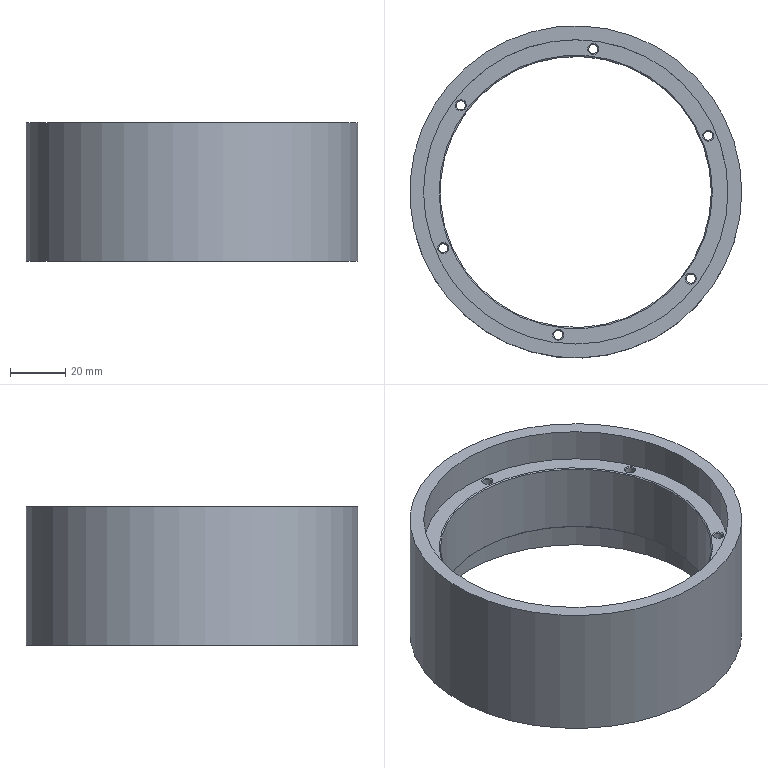Part | NX | features Instance Feature 6, SYMBOLIC_THREAD 6, DATUM_CSYS 5, IDENTICAL INSTANCE OUTPUT 5, EXTRUDE 4, SKETCH 4, EXTRACT_FACE 2, EXTRACT_STRING 2, CHAMFER 1, DATUM_PLANE 1, HOLE PACKAGE 1, MASTER SNAPSHOT BODY 1, Mirror Feature 1, Pattern Feature 1, SIMPLE HOLE 1 | 1 solid | 28 faces | box 120 x 120 x 50 mm | volume 139903 mm3 | cone 14 | cylinder 10 | plane 4 | commonest cylinder face diameters 3.3 x6 110 x2 98 x1 120 x1
STEP:
#1=CARTESIAN_POINT('',(60.,0.,-50.));
#2=VERTEX_POINT('',#1);
#3=CARTESIAN_POINT('',(0.,0.,-50.));
#4=DIRECTION('',(0.,0.,1.));
#5=DIRECTION('',(1.,0.,0.));
#6=AXIS2_PLACEMENT_3D('',#3,#4,#5);
#7=CIRCLE('',#6,60.);
#8=EDGE_CURVE('',#2,#2,#7,.T.);
#9=ORIENTED_EDGE('',*,*,#8,.T.);
#10=EDGE_LOOP('',(#9));
#11=FACE_BOUND('',#10,.T.);
#12=CARTESIAN_POINT('',(60.,0.,0.));
#13=VERTEX_POINT('',#12);
#14=CARTESIAN_POINT('',(0.,0.,0.));
#15=DIRECTION('',(0.,0.,1.));
#16=DIRECTION('',(1.,0.,0.));
#17=AXIS2_PLACEMENT_3D('',#14,#15,#16);
#18=CIRCLE('',#17,60.);
#19=EDGE_CURVE('',#13,#13,#18,.T.);
#20=ORIENTED_EDGE('',*,*,#19,.F.);
#21=EDGE_LOOP('',(#20));
#22=FACE_BOUND('',#21,.T.);
#23=CARTESIAN_POINT('',(0.,0.,-50.));
#24=DIRECTION('',(0.,0.,1.));
#25=DIRECTION('',(1.,0.,0.));
#26=AXIS2_PLACEMENT_3D('',#23,#24,#25);
#27=CYLINDRICAL_SURFACE('',#26,60.);
#28=ADVANCED_FACE('',(#11,#22),#27,.T.);
#29=CARTESIAN_POINT('',(55.,0.,-50.));
#30=VERTEX_POINT('',#29);
#31=CARTESIAN_POINT('',(0.,0.,-50.));
#32=DIRECTION('',(0.,0.,1.));
#33=DIRECTION('',(1.,0.,0.));
#34=AXIS2_PLACEMENT_3D('',#31,#32,#33);
#35=CIRCLE('',#34,55.);
#36=EDGE_CURVE('',#30,#30,#35,.T.);
#37=ORIENTED_EDGE('',*,*,#36,.T.);
#38=EDGE_LOOP('',(#37));
#39=FACE_BOUND('',#38,.T.);
#40=ORIENTED_EDGE('',*,*,#8,.F.);
#41=EDGE_LOOP('',(#40));
#42=FACE_BOUND('',#41,.T.);
#43=CARTESIAN_POINT('',(0.,0.,-50.));
#44=DIRECTION('',(0.,0.,1.));
#45=DIRECTION('',(1.,0.,0.));
#46=AXIS2_PLACEMENT_3D('',#43,#44,#45);
#47=PLANE('',#46);
#48=ADVANCED_FACE('',(#39,#42),#47,.F.);
#49=CARTESIAN_POINT('',(55.,0.,0.));
#50=VERTEX_POINT('',#49);
#51=CARTESIAN_POINT('',(0.,0.,0.));
#52=DIRECTION('',(0.,0.,1.));
#53=DIRECTION('',(1.,0.,0.));
#54=AXIS2_PLACEMENT_3D('',#51,#52,#53);
#55=CIRCLE('',#54,55.);
#56=EDGE_CURVE('',#50,#50,#55,.T.);
#57=ORIENTED_EDGE('',*,*,#56,.F.);
#58=EDGE_LOOP('',(#57));
#59=FACE_BOUND('',#58,.T.);
#60=ORIENTED_EDGE('',*,*,#19,.T.);
#61=EDGE_LOOP('',(#60));
#62=FACE_BOUND('',#61,.T.);
#63=CARTESIAN_POINT('',(0.,0.,0.));
#64=DIRECTION('',(0.,0.,1.));
#65=DIRECTION('',(1.,0.,0.));
#66=AXIS2_PLACEMENT_3D('',#63,#64,#65);
#67=PLANE('',#66);
#68=ADVANCED_FACE('',(#59,#62),#67,.T.);
#69=CARTESIAN_POINT('',(55.,0.,-12.));
#70=VERTEX_POINT('',#69);
#71=CARTESIAN_POINT('',(0.,0.,-12.));
#72=DIRECTION('',(0.,0.,1.));
#73=DIRECTION('',(1.,0.,0.));
#74=AXIS2_PLACEMENT_3D('',#71,#72,#73);
#75=CIRCLE('',#74,55.);
#76=EDGE_CURVE('',#70,#70,#75,.F.);
#77=ORIENTED_EDGE('',*,*,#76,.T.);
#78=EDGE_LOOP('',(#77));
#79=FACE_BOUND('',#78,.T.);
#80=ORIENTED_EDGE('',*,*,#56,.T.);
#81=EDGE_LOOP('',(#80));
#82=FACE_BOUND('',#81,.T.);
#83=CARTESIAN_POINT('',(0.,0.,-12.));
#84=DIRECTION('',(0.,0.,1.));
#85=DIRECTION('',(1.,0.,0.));
#86=AXIS2_PLACEMENT_3D('',#83,#84,#85);
#87=CYLINDRICAL_SURFACE('',#86,55.);
#88=ADVANCED_FACE('',(#79,#82),#87,.F.);
#89=CARTESIAN_POINT('',(49.38,0.,-12.));
#90=VERTEX_POINT('',#89);
#91=CARTESIAN_POINT('',(0.,0.,-12.));
#92=DIRECTION('',(0.,0.,1.));
#93=DIRECTION('',(1.,0.,0.));
#94=AXIS2_PLACEMENT_3D('',#91,#92,#93);
#95=CIRCLE('',#94,49.38);
#96=EDGE_CURVE('',#90,#90,#95,.F.);
#97=ORIENTED_EDGE('',*,*,#96,.T.);
#98=EDGE_LOOP('',(#97));
#99=FACE_BOUND('',#98,.T.);
#100=CARTESIAN_POINT('',(8.337,51.612,-12.));
#101=VERTEX_POINT('',#100);
#102=CARTESIAN_POINT('',(6.337,51.612,-12.));
#103=DIRECTION('',(0.,0.,1.));
#104=DIRECTION('',(1.,0.,0.));
#105=AXIS2_PLACEMENT_3D('',#102,#103,#104);
#106=CIRCLE('',#105,2.);
#107=EDGE_CURVE('',#101,#101,#106,.T.);
#108=ORIENTED_EDGE('',*,*,#107,.F.);
#109=EDGE_LOOP('',(#108));
#110=FACE_BOUND('',#109,.T.);
#111=CARTESIAN_POINT('',(49.866,20.318,-12.));
#112=VERTEX_POINT('',#111);
#113=CARTESIAN_POINT('',(47.866,20.318,-12.));
#114=DIRECTION('',(0.,0.,1.));
#115=DIRECTION('',(1.,0.,0.));
#116=AXIS2_PLACEMENT_3D('',#113,#114,#115);
#117=CIRCLE('',#116,2.);
#118=EDGE_CURVE('',#112,#112,#117,.T.);
#119=ORIENTED_EDGE('',*,*,#118,.F.);
#120=EDGE_LOOP('',(#119));
#121=FACE_BOUND('',#120,.T.);
#122=CARTESIAN_POINT('',(43.529,-31.294,-12.));
#123=VERTEX_POINT('',#122);
#124=CARTESIAN_POINT('',(41.529,-31.294,-12.));
#125=DIRECTION('',(0.,0.,1.));
#126=DIRECTION('',(1.,0.,0.));
#127=AXIS2_PLACEMENT_3D('',#124,#125,#126);
#128=CIRCLE('',#127,2.);
#129=EDGE_CURVE('',#123,#123,#128,.T.);
#130=ORIENTED_EDGE('',*,*,#129,.F.);
#131=EDGE_LOOP('',(#130));
#132=FACE_BOUND('',#131,.T.);
#133=CARTESIAN_POINT('',(-4.337,-51.612,-12.));
#134=VERTEX_POINT('',#133);
#135=CARTESIAN_POINT('',(-6.337,-51.612,-12.));
#136=DIRECTION('',(0.,0.,1.));
#137=DIRECTION('',(1.,0.,0.));
#138=AXIS2_PLACEMENT_3D('',#135,#136,#137);
#139=CIRCLE('',#138,2.);
#140=EDGE_CURVE('',#134,#134,#139,.T.);
#141=ORIENTED_EDGE('',*,*,#140,.F.);
#142=EDGE_LOOP('',(#141));
#143=FACE_BOUND('',#142,.T.);
#144=CARTESIAN_POINT('',(-45.866,-20.318,-12.));
#145=VERTEX_POINT('',#144);
#146=CARTESIAN_POINT('',(-47.866,-20.318,-12.));
#147=DIRECTION('',(0.,0.,1.));
#148=DIRECTION('',(1.,0.,0.));
#149=AXIS2_PLACEMENT_3D('',#146,#147,#148);
#150=CIRCLE('',#149,2.);
#151=EDGE_CURVE('',#145,#145,#150,.T.);
#152=ORIENTED_EDGE('',*,*,#151,.F.);
#153=EDGE_LOOP('',(#152));
#154=FACE_BOUND('',#153,.T.);
#155=CARTESIAN_POINT('',(-39.529,31.294,-12.));
#156=VERTEX_POINT('',#155);
#157=CARTESIAN_POINT('',(-41.529,31.294,-12.));
#158=DIRECTION('',(0.,0.,1.));
#159=DIRECTION('',(1.,0.,0.));
#160=AXIS2_PLACEMENT_3D('',#157,#158,#159);
#161=CIRCLE('',#160,2.);
#162=EDGE_CURVE('',#156,#156,#161,.T.);
#163=ORIENTED_EDGE('',*,*,#162,.F.);
#164=EDGE_LOOP('',(#163));
#165=FACE_BOUND('',#164,.T.);
#166=ORIENTED_EDGE('',*,*,#76,.F.);
#167=EDGE_LOOP('',(#166));
#168=FACE_BOUND('',#167,.T.);
#169=CARTESIAN_POINT('',(0.,0.,-12.));
#170=DIRECTION('',(0.,0.,1.));
#171=DIRECTION('',(1.,0.,0.));
#172=AXIS2_PLACEMENT_3D('',#169,#170,#171);
#173=PLANE('',#172);
#174=ADVANCED_FACE('',(#99,#110,#121,#132,#143,#154,#165,#168),#173,.T.);
#175=CARTESIAN_POINT('',(55.,0.,-38.));
#176=VERTEX_POINT('',#175);
#177=CARTESIAN_POINT('',(0.,0.,-38.));
#178=DIRECTION('',(0.,0.,1.));
#179=DIRECTION('',(1.,0.,0.));
#180=AXIS2_PLACEMENT_3D('',#177,#178,#179);
#181=CIRCLE('',#180,55.);
#182=EDGE_CURVE('',#176,#176,#181,.F.);
#183=ORIENTED_EDGE('',*,*,#182,.F.);
#184=EDGE_LOOP('',(#183));
#185=FACE_BOUND('',#184,.T.);
#186=ORIENTED_EDGE('',*,*,#36,.F.);
#187=EDGE_LOOP('',(#186));
#188=FACE_BOUND('',#187,.T.);
#189=CARTESIAN_POINT('',(0.,0.,-38.));
#190=DIRECTION('',(0.,0.,-1.));
#191=DIRECTION('',(-1.,0.,0.));
#192=AXIS2_PLACEMENT_3D('',#189,#190,#191);
#193=CYLINDRICAL_SURFACE('',#192,55.);
#194=ADVANCED_FACE('',(#185,#188),#193,.F.);
#195=CARTESIAN_POINT('',(49.38,0.,-38.));
#196=VERTEX_POINT('',#195);
#197=CARTESIAN_POINT('',(0.,0.,-38.));
#198=DIRECTION('',(0.,0.,1.));
#199=DIRECTION('',(1.,0.,0.));
#200=AXIS2_PLACEMENT_3D('',#197,#198,#199);
#201=CIRCLE('',#200,49.38);
#202=EDGE_CURVE('',#196,#196,#201,.T.);
#203=ORIENTED_EDGE('',*,*,#202,.T.);
#204=EDGE_LOOP('',(#203));
#205=FACE_BOUND('',#204,.T.);
#206=CARTESIAN_POINT('',(8.337,51.612,-38.));
#207=VERTEX_POINT('',#206);
#208=CARTESIAN_POINT('',(6.337,51.612,-38.));
#209=DIRECTION('',(0.,0.,1.));
#210=DIRECTION('',(1.,0.,0.));
#211=AXIS2_PLACEMENT_3D('',#208,#209,#210);
#212=CIRCLE('',#211,2.);
#213=EDGE_CURVE('',#207,#207,#212,.T.);
#214=ORIENTED_EDGE('',*,*,#213,.T.);
#215=EDGE_LOOP('',(#214));
#216=FACE_BOUND('',#215,.T.);
#217=CARTESIAN_POINT('',(49.866,20.318,-38.));
#218=VERTEX_POINT('',#217);
#219=CARTESIAN_POINT('',(47.866,20.318,-38.));
#220=DIRECTION('',(0.,0.,1.));
#221=DIRECTION('',(1.,0.,0.));
#222=AXIS2_PLACEMENT_3D('',#219,#220,#221);
#223=CIRCLE('',#222,2.);
#224=EDGE_CURVE('',#218,#218,#223,.T.);
#225=ORIENTED_EDGE('',*,*,#224,.T.);
#226=EDGE_LOOP('',(#225));
#227=FACE_BOUND('',#226,.T.);
#228=CARTESIAN_POINT('',(43.529,-31.294,-38.));
#229=VERTEX_POINT('',#228);
#230=CARTESIAN_POINT('',(41.529,-31.294,-38.));
#231=DIRECTION('',(0.,0.,1.));
#232=DIRECTION('',(1.,0.,0.));
#233=AXIS2_PLACEMENT_3D('',#230,#231,#232);
#234=CIRCLE('',#233,2.);
#235=EDGE_CURVE('',#229,#229,#234,.T.);
#236=ORIENTED_EDGE('',*,*,#235,.T.);
#237=EDGE_LOOP('',(#236));
#238=FACE_BOUND('',#237,.T.);
#239=CARTESIAN_POINT('',(-4.337,-51.612,-38.));
#240=VERTEX_POINT('',#239);
#241=CARTESIAN_POINT('',(-6.337,-51.612,-38.));
#242=DIRECTION('',(0.,0.,1.));
#243=DIRECTION('',(1.,0.,0.));
#244=AXIS2_PLACEMENT_3D('',#241,#242,#243);
#245=CIRCLE('',#244,2.);
#246=EDGE_CURVE('',#240,#240,#245,.T.);
#247=ORIENTED_EDGE('',*,*,#246,.T.);
#248=EDGE_LOOP('',(#247));
#249=FACE_BOUND('',#248,.T.);
#250=CARTESIAN_POINT('',(-45.866,-20.318,-38.));
#251=VERTEX_POINT('',#250);
#252=CARTESIAN_POINT('',(-47.866,-20.318,-38.));
#253=DIRECTION('',(0.,0.,1.));
#254=DIRECTION('',(1.,0.,0.));
#255=AXIS2_PLACEMENT_3D('',#252,#253,#254);
#256=CIRCLE('',#255,2.);
#257=EDGE_CURVE('',#251,#251,#256,.T.);
#258=ORIENTED_EDGE('',*,*,#257,.T.);
#259=EDGE_LOOP('',(#258));
#260=FACE_BOUND('',#259,.T.);
#261=CARTESIAN_POINT('',(-39.529,31.294,-38.));
#262=VERTEX_POINT('',#261);
#263=CARTESIAN_POINT('',(-41.529,31.294,-38.));
#264=DIRECTION('',(0.,0.,1.));
#265=DIRECTION('',(1.,0.,0.));
#266=AXIS2_PLACEMENT_3D('',#263,#264,#265);
#267=CIRCLE('',#266,2.);
#268=EDGE_CURVE('',#262,#262,#267,.T.);
#269=ORIENTED_EDGE('',*,*,#268,.T.);
#270=EDGE_LOOP('',(#269));
#271=FACE_BOUND('',#270,.T.);
#272=ORIENTED_EDGE('',*,*,#182,.T.);
#273=EDGE_LOOP('',(#272));
#274=FACE_BOUND('',#273,.T.);
#275=CARTESIAN_POINT('',(0.,0.,-38.));
#276=DIRECTION('',(0.,0.,1.));
#277=DIRECTION('',(1.,0.,0.));
#278=AXIS2_PLACEMENT_3D('',#275,#276,#277);
#279=PLANE('',#278);
#280=ADVANCED_FACE('',(#205,#216,#227,#238,#249,#260,#271,#274),#279,.F.);
#281=CARTESIAN_POINT('',(49.,0.,-37.62));
#282=VERTEX_POINT('',#281);
#283=CARTESIAN_POINT('',(0.,0.,-37.62));
#284=DIRECTION('',(0.,0.,1.));
#285=DIRECTION('',(1.,0.,0.));
#286=AXIS2_PLACEMENT_3D('',#283,#284,#285);
#287=CIRCLE('',#286,49.);
#288=EDGE_CURVE('',#282,#282,#287,.F.);
#289=ORIENTED_EDGE('',*,*,#288,.T.);
#290=EDGE_LOOP('',(#289));
#291=FACE_BOUND('',#290,.T.);
#292=CARTESIAN_POINT('',(49.,0.,-12.38));
#293=VERTEX_POINT('',#292);
#294=CARTESIAN_POINT('',(0.,0.,-12.38));
#295=DIRECTION('',(0.,0.,1.));
#296=DIRECTION('',(1.,0.,0.));
#297=AXIS2_PLACEMENT_3D('',#294,#295,#296);
#298=CIRCLE('',#297,49.);
#299=EDGE_CURVE('',#293,#293,#298,.T.);
#300=ORIENTED_EDGE('',*,*,#299,.T.);
#301=EDGE_LOOP('',(#300));
#302=FACE_BOUND('',#301,.T.);
#303=CARTESIAN_POINT('',(0.,0.,-102.));
#304=DIRECTION('',(0.,0.,1.));
#305=DIRECTION('',(1.,0.,0.));
#306=AXIS2_PLACEMENT_3D('',#303,#304,#305);
#307=CYLINDRICAL_SURFACE('',#306,49.);
#308=ADVANCED_FACE('',(#291,#302),#307,.F.);
#309=CARTESIAN_POINT('',(-43.179,31.294,-37.65));
#310=VERTEX_POINT('',#309);
#311=CARTESIAN_POINT('',(-41.529,31.294,-37.65));
#312=DIRECTION('',(0.,0.,-1.));
#313=DIRECTION('',(-1.,0.,0.));
#314=AXIS2_PLACEMENT_3D('',#311,#312,#313);
#315=CIRCLE('',#314,1.65);
#316=EDGE_CURVE('',#310,#310,#315,.T.);
#317=ORIENTED_EDGE('',*,*,#316,.T.);
#318=EDGE_LOOP('',(#317));
#319=FACE_BOUND('',#318,.T.);
#320=CARTESIAN_POINT('',(-39.879,31.294,-12.35));
#321=VERTEX_POINT('',#320);
#322=CARTESIAN_POINT('',(-41.529,31.294,-12.35));
#323=DIRECTION('',(0.,0.,1.));
#324=DIRECTION('',(1.,0.,0.));
#325=AXIS2_PLACEMENT_3D('',#322,#323,#324);
#326=CIRCLE('',#325,1.65);
#327=EDGE_CURVE('',#321,#321,#326,.T.);
#328=ORIENTED_EDGE('',*,*,#327,.T.);
#329=EDGE_LOOP('',(#328));
#330=FACE_BOUND('',#329,.T.);
#331=CARTESIAN_POINT('',(-41.529,31.294,-12.));
#332=DIRECTION('',(0.,0.,-1.));
#333=DIRECTION('',(-1.,0.,0.));
#334=AXIS2_PLACEMENT_3D('',#331,#332,#333);
#335=CYLINDRICAL_SURFACE('',#334,1.65);
#336=ADVANCED_FACE('',(#319,#330),#335,.F.);
#337=ORIENTED_EDGE('',*,*,#162,.T.);
#338=EDGE_LOOP('',(#337));
#339=FACE_BOUND('',#338,.T.);
#340=ORIENTED_EDGE('',*,*,#327,.F.);
#341=EDGE_LOOP('',(#340));
#342=FACE_BOUND('',#341,.T.);
#343=CARTESIAN_POINT('',(-41.529,31.294,-14.));
#344=DIRECTION('',(0.,0.,1.));
#345=DIRECTION('',(1.,0.,0.));
#346=AXIS2_PLACEMENT_3D('',#343,#344,#345);
#347=CONICAL_SURFACE('',#346,0.,0.7854);
#348=ADVANCED_FACE('',(#339,#342),#347,.F.);
#349=ORIENTED_EDGE('',*,*,#316,.F.);
#350=EDGE_LOOP('',(#349));
#351=FACE_BOUND('',#350,.T.);
#352=ORIENTED_EDGE('',*,*,#268,.F.);
#353=EDGE_LOOP('',(#352));
#354=FACE_BOUND('',#353,.T.);
#355=CARTESIAN_POINT('',(-41.529,31.294,-36.));
#356=DIRECTION('',(0.,0.,-1.));
#357=DIRECTION('',(-1.,0.,0.));
#358=AXIS2_PLACEMENT_3D('',#355,#356,#357);
#359=CONICAL_SURFACE('',#358,0.,0.7854);
#360=ADVANCED_FACE('',(#351,#354),#359,.F.);
#361=CARTESIAN_POINT('',(4.687,51.612,-37.65));
#362=VERTEX_POINT('',#361);
#363=CARTESIAN_POINT('',(6.337,51.612,-37.65));
#364=DIRECTION('',(0.,0.,-1.));
#365=DIRECTION('',(-1.,0.,0.));
#366=AXIS2_PLACEMENT_3D('',#363,#364,#365);
#367=CIRCLE('',#366,1.65);
#368=EDGE_CURVE('',#362,#362,#367,.T.);
#369=ORIENTED_EDGE('',*,*,#368,.T.);
#370=EDGE_LOOP('',(#369));
#371=FACE_BOUND('',#370,.T.);
#372=CARTESIAN_POINT('',(7.987,51.612,-12.35));
#373=VERTEX_POINT('',#372);
#374=CARTESIAN_POINT('',(6.337,51.612,-12.35));
#375=DIRECTION('',(0.,0.,1.));
#376=DIRECTION('',(1.,0.,0.));
#377=AXIS2_PLACEMENT_3D('',#374,#375,#376);
#378=CIRCLE('',#377,1.65);
#379=EDGE_CURVE('',#373,#373,#378,.T.);
#380=ORIENTED_EDGE('',*,*,#379,.T.);
#381=EDGE_LOOP('',(#380));
#382=FACE_BOUND('',#381,.T.);
#383=CARTESIAN_POINT('',(6.337,51.612,-12.));
#384=DIRECTION('',(0.,0.,-1.));
#385=DIRECTION('',(-0.5,0.866,0.));
#386=AXIS2_PLACEMENT_3D('',#383,#384,#385);
#387=CYLINDRICAL_SURFACE('',#386,1.65);
#388=ADVANCED_FACE('',(#371,#382),#387,.F.);
#389=CARTESIAN_POINT('',(46.216,20.318,-37.65));
#390=VERTEX_POINT('',#389);
#391=CARTESIAN_POINT('',(47.866,20.318,-37.65));
#392=DIRECTION('',(0.,0.,-1.));
#393=DIRECTION('',(-1.,0.,0.));
#394=AXIS2_PLACEMENT_3D('',#391,#392,#393);
#395=CIRCLE('',#394,1.65);
#396=EDGE_CURVE('',#390,#390,#395,.T.);
#397=ORIENTED_EDGE('',*,*,#396,.T.);
#398=EDGE_LOOP('',(#397));
#399=FACE_BOUND('',#398,.T.);
#400=CARTESIAN_POINT('',(49.516,20.318,-12.35));
#401=VERTEX_POINT('',#400);
#402=CARTESIAN_POINT('',(47.866,20.318,-12.35));
#403=DIRECTION('',(0.,0.,1.));
#404=DIRECTION('',(1.,0.,0.));
#405=AXIS2_PLACEMENT_3D('',#402,#403,#404);
#406=CIRCLE('',#405,1.65);
#407=EDGE_CURVE('',#401,#401,#406,.T.);
#408=ORIENTED_EDGE('',*,*,#407,.T.);
#409=EDGE_LOOP('',(#408));
#410=FACE_BOUND('',#409,.T.);
#411=CARTESIAN_POINT('',(47.866,20.318,-12.));
#412=DIRECTION('',(0.,0.,-1.));
#413=DIRECTION('',(0.5,0.866,0.));
#414=AXIS2_PLACEMENT_3D('',#411,#412,#413);
#415=CYLINDRICAL_SURFACE('',#414,1.65);
#416=ADVANCED_FACE('',(#399,#410),#415,.F.);
#417=CARTESIAN_POINT('',(39.879,-31.294,-37.65));
#418=VERTEX_POINT('',#417);
#419=CARTESIAN_POINT('',(41.529,-31.294,-37.65));
#420=DIRECTION('',(0.,0.,-1.));
#421=DIRECTION('',(-1.,0.,0.));
#422=AXIS2_PLACEMENT_3D('',#419,#420,#421);
#423=CIRCLE('',#422,1.65);
#424=EDGE_CURVE('',#418,#418,#423,.T.);
#425=ORIENTED_EDGE('',*,*,#424,.T.);
#426=EDGE_LOOP('',(#425));
#427=FACE_BOUND('',#426,.T.);
#428=CARTESIAN_POINT('',(43.179,-31.294,-12.35));
#429=VERTEX_POINT('',#428);
#430=CARTESIAN_POINT('',(41.529,-31.294,-12.35));
#431=DIRECTION('',(0.,0.,1.));
#432=DIRECTION('',(1.,0.,0.));
#433=AXIS2_PLACEMENT_3D('',#430,#431,#432);
#434=CIRCLE('',#433,1.65);
#435=EDGE_CURVE('',#429,#429,#434,.T.);
#436=ORIENTED_EDGE('',*,*,#435,.T.);
#437=EDGE_LOOP('',(#436));
#438=FACE_BOUND('',#437,.T.);
#439=CARTESIAN_POINT('',(41.529,-31.294,-12.));
#440=DIRECTION('',(0.,0.,-1.));
#441=DIRECTION('',(1.,0.,0.));
#442=AXIS2_PLACEMENT_3D('',#439,#440,#441);
#443=CYLINDRICAL_SURFACE('',#442,1.65);
#444=ADVANCED_FACE('',(#427,#438),#443,.F.);
#445=CARTESIAN_POINT('',(-7.987,-51.612,-37.65));
#446=VERTEX_POINT('',#445);
#447=CARTESIAN_POINT('',(-6.337,-51.612,-37.65));
#448=DIRECTION('',(0.,0.,-1.));
#449=DIRECTION('',(-1.,0.,0.));
#450=AXIS2_PLACEMENT_3D('',#447,#448,#449);
#451=CIRCLE('',#450,1.65);
#452=EDGE_CURVE('',#446,#446,#451,.T.);
#453=ORIENTED_EDGE('',*,*,#452,.T.);
#454=EDGE_LOOP('',(#453));
#455=FACE_BOUND('',#454,.T.);
#456=CARTESIAN_POINT('',(-4.687,-51.612,-12.35));
#457=VERTEX_POINT('',#456);
#458=CARTESIAN_POINT('',(-6.337,-51.612,-12.35));
#459=DIRECTION('',(0.,0.,1.));
#460=DIRECTION('',(1.,0.,0.));
#461=AXIS2_PLACEMENT_3D('',#458,#459,#460);
#462=CIRCLE('',#461,1.65);
#463=EDGE_CURVE('',#457,#457,#462,.T.);
#464=ORIENTED_EDGE('',*,*,#463,.T.);
#465=EDGE_LOOP('',(#464));
#466=FACE_BOUND('',#465,.T.);
#467=CARTESIAN_POINT('',(-6.337,-51.612,-12.));
#468=DIRECTION('',(0.,0.,-1.));
#469=DIRECTION('',(0.5,-0.866,0.));
#470=AXIS2_PLACEMENT_3D('',#467,#468,#469);
#471=CYLINDRICAL_SURFACE('',#470,1.65);
#472=ADVANCED_FACE('',(#455,#466),#471,.F.);
#473=CARTESIAN_POINT('',(-49.516,-20.318,-37.65));
#474=VERTEX_POINT('',#473);
#475=CARTESIAN_POINT('',(-47.866,-20.318,-37.65));
#476=DIRECTION('',(0.,0.,-1.));
#477=DIRECTION('',(-1.,0.,0.));
#478=AXIS2_PLACEMENT_3D('',#475,#476,#477);
#479=CIRCLE('',#478,1.65);
#480=EDGE_CURVE('',#474,#474,#479,.T.);
#481=ORIENTED_EDGE('',*,*,#480,.T.);
#482=EDGE_LOOP('',(#481));
#483=FACE_BOUND('',#482,.T.);
#484=CARTESIAN_POINT('',(-46.216,-20.318,-12.35));
#485=VERTEX_POINT('',#484);
#486=CARTESIAN_POINT('',(-47.866,-20.318,-12.35));
#487=DIRECTION('',(0.,0.,1.));
#488=DIRECTION('',(1.,0.,0.));
#489=AXIS2_PLACEMENT_3D('',#486,#487,#488);
#490=CIRCLE('',#489,1.65);
#491=EDGE_CURVE('',#485,#485,#490,.T.);
#492=ORIENTED_EDGE('',*,*,#491,.T.);
#493=EDGE_LOOP('',(#492));
#494=FACE_BOUND('',#493,.T.);
#495=CARTESIAN_POINT('',(-47.866,-20.318,-12.));
#496=DIRECTION('',(0.,0.,-1.));
#497=DIRECTION('',(-0.5,-0.866,0.));
#498=AXIS2_PLACEMENT_3D('',#495,#496,#497);
#499=CYLINDRICAL_SURFACE('',#498,1.65);
#500=ADVANCED_FACE('',(#483,#494),#499,.F.);
#501=ORIENTED_EDGE('',*,*,#151,.T.);
#502=EDGE_LOOP('',(#501));
#503=FACE_BOUND('',#502,.T.);
#504=ORIENTED_EDGE('',*,*,#491,.F.);
#505=EDGE_LOOP('',(#504));
#506=FACE_BOUND('',#505,.T.);
#507=CARTESIAN_POINT('',(-47.866,-20.318,-14.));
#508=DIRECTION('',(0.,0.,1.));
#509=DIRECTION('',(1.,0.,0.));
#510=AXIS2_PLACEMENT_3D('',#507,#508,#509);
#511=CONICAL_SURFACE('',#510,0.,0.7854);
#512=ADVANCED_FACE('',(#503,#506),#511,.F.);
#513=ORIENTED_EDGE('',*,*,#140,.T.);
#514=EDGE_LOOP('',(#513));
#515=FACE_BOUND('',#514,.T.);
#516=ORIENTED_EDGE('',*,*,#463,.F.);
#517=EDGE_LOOP('',(#516));
#518=FACE_BOUND('',#517,.T.);
#519=CARTESIAN_POINT('',(-6.337,-51.612,-14.));
#520=DIRECTION('',(0.,0.,1.));
#521=DIRECTION('',(1.,0.,0.));
#522=AXIS2_PLACEMENT_3D('',#519,#520,#521);
#523=CONICAL_SURFACE('',#522,0.,0.7854);
#524=ADVANCED_FACE('',(#515,#518),#523,.F.);
#525=ORIENTED_EDGE('',*,*,#129,.T.);
#526=EDGE_LOOP('',(#525));
#527=FACE_BOUND('',#526,.T.);
#528=ORIENTED_EDGE('',*,*,#435,.F.);
#529=EDGE_LOOP('',(#528));
#530=FACE_BOUND('',#529,.T.);
#531=CARTESIAN_POINT('',(41.529,-31.294,-14.));
#532=DIRECTION('',(0.,0.,1.));
#533=DIRECTION('',(1.,0.,0.));
#534=AXIS2_PLACEMENT_3D('',#531,#532,#533);
#535=CONICAL_SURFACE('',#534,0.,0.7854);
#536=ADVANCED_FACE('',(#527,#530),#535,.F.);
#537=ORIENTED_EDGE('',*,*,#118,.T.);
#538=EDGE_LOOP('',(#537));
#539=FACE_BOUND('',#538,.T.);
#540=ORIENTED_EDGE('',*,*,#407,.F.);
#541=EDGE_LOOP('',(#540));
#542=FACE_BOUND('',#541,.T.);
#543=CARTESIAN_POINT('',(47.866,20.318,-14.));
#544=DIRECTION('',(0.,0.,1.));
#545=DIRECTION('',(1.,0.,0.));
#546=AXIS2_PLACEMENT_3D('',#543,#544,#545);
#547=CONICAL_SURFACE('',#546,0.,0.7854);
#548=ADVANCED_FACE('',(#539,#542),#547,.F.);
#549=ORIENTED_EDGE('',*,*,#107,.T.);
#550=EDGE_LOOP('',(#549));
#551=FACE_BOUND('',#550,.T.);
#552=ORIENTED_EDGE('',*,*,#379,.F.);
#553=EDGE_LOOP('',(#552));
#554=FACE_BOUND('',#553,.T.);
#555=CARTESIAN_POINT('',(6.337,51.612,-14.));
#556=DIRECTION('',(0.,0.,1.));
#557=DIRECTION('',(1.,0.,0.));
#558=AXIS2_PLACEMENT_3D('',#555,#556,#557);
#559=CONICAL_SURFACE('',#558,0.,0.7854);
#560=ADVANCED_FACE('',(#551,#554),#559,.F.);
#561=ORIENTED_EDGE('',*,*,#480,.F.);
#562=EDGE_LOOP('',(#561));
#563=FACE_BOUND('',#562,.T.);
#564=ORIENTED_EDGE('',*,*,#257,.F.);
#565=EDGE_LOOP('',(#564));
#566=FACE_BOUND('',#565,.T.);
#567=CARTESIAN_POINT('',(-47.866,-20.318,-36.));
#568=DIRECTION('',(0.,0.,-1.));
#569=DIRECTION('',(-1.,0.,0.));
#570=AXIS2_PLACEMENT_3D('',#567,#568,#569);
#571=CONICAL_SURFACE('',#570,0.,0.7854);
#572=ADVANCED_FACE('',(#563,#566),#571,.F.);
#573=ORIENTED_EDGE('',*,*,#246,.F.);
#574=EDGE_LOOP('',(#573));
#575=FACE_BOUND('',#574,.T.);
#576=ORIENTED_EDGE('',*,*,#452,.F.);
#577=EDGE_LOOP('',(#576));
#578=FACE_BOUND('',#577,.T.);
#579=CARTESIAN_POINT('',(-6.337,-51.612,-36.));
#580=DIRECTION('',(0.,0.,-1.));
#581=DIRECTION('',(-1.,0.,0.));
#582=AXIS2_PLACEMENT_3D('',#579,#580,#581);
#583=CONICAL_SURFACE('',#582,0.,0.7854);
#584=ADVANCED_FACE('',(#575,#578),#583,.F.);
#585=ORIENTED_EDGE('',*,*,#235,.F.);
#586=EDGE_LOOP('',(#585));
#587=FACE_BOUND('',#586,.T.);
#588=ORIENTED_EDGE('',*,*,#424,.F.);
#589=EDGE_LOOP('',(#588));
#590=FACE_BOUND('',#589,.T.);
#591=CARTESIAN_POINT('',(41.529,-31.294,-36.));
#592=DIRECTION('',(0.,0.,-1.));
#593=DIRECTION('',(-1.,0.,0.));
#594=AXIS2_PLACEMENT_3D('',#591,#592,#593);
#595=CONICAL_SURFACE('',#594,0.,0.7854);
#596=ADVANCED_FACE('',(#587,#590),#595,.F.);
#597=ORIENTED_EDGE('',*,*,#224,.F.);
#598=EDGE_LOOP('',(#597));
#599=FACE_BOUND('',#598,.T.);
#600=ORIENTED_EDGE('',*,*,#396,.F.);
#601=EDGE_LOOP('',(#600));
#602=FACE_BOUND('',#601,.T.);
#603=CARTESIAN_POINT('',(47.866,20.318,-36.));
#604=DIRECTION('',(0.,0.,-1.));
#605=DIRECTION('',(-1.,0.,0.));
#606=AXIS2_PLACEMENT_3D('',#603,#604,#605);
#607=CONICAL_SURFACE('',#606,0.,0.7854);
#608=ADVANCED_FACE('',(#599,#602),#607,.F.);
#609=ORIENTED_EDGE('',*,*,#213,.F.);
#610=EDGE_LOOP('',(#609));
#611=FACE_BOUND('',#610,.T.);
#612=ORIENTED_EDGE('',*,*,#368,.F.);
#613=EDGE_LOOP('',(#612));
#614=FACE_BOUND('',#613,.T.);
#615=CARTESIAN_POINT('',(6.337,51.612,-36.));
#616=DIRECTION('',(0.,0.,-1.));
#617=DIRECTION('',(-1.,0.,0.));
#618=AXIS2_PLACEMENT_3D('',#615,#616,#617);
#619=CONICAL_SURFACE('',#618,0.,0.7854);
#620=ADVANCED_FACE('',(#611,#614),#619,.F.);
#621=ORIENTED_EDGE('',*,*,#288,.F.);
#622=EDGE_LOOP('',(#621));
#623=FACE_BOUND('',#622,.T.);
#624=ORIENTED_EDGE('',*,*,#202,.F.);
#625=EDGE_LOOP('',(#624));
#626=FACE_BOUND('',#625,.T.);
#627=CARTESIAN_POINT('',(0.,0.,-38.));
#628=DIRECTION('',(0.,0.,-1.));
#629=DIRECTION('',(-1.,0.,0.));
#630=AXIS2_PLACEMENT_3D('',#627,#628,#629);
#631=CONICAL_SURFACE('',#630,49.38,0.7854);
#632=ADVANCED_FACE('',(#623,#626),#631,.F.);
#633=ORIENTED_EDGE('',*,*,#96,.F.);
#634=EDGE_LOOP('',(#633));
#635=FACE_BOUND('',#634,.T.);
#636=ORIENTED_EDGE('',*,*,#299,.F.);
#637=EDGE_LOOP('',(#636));
#638=FACE_BOUND('',#637,.T.);
#639=CARTESIAN_POINT('',(0.,0.,-12.38));
#640=DIRECTION('',(0.,0.,1.));
#641=DIRECTION('',(1.,0.,0.));
#642=AXIS2_PLACEMENT_3D('',#639,#640,#641);
#643=CONICAL_SURFACE('',#642,49.,0.7854);
#644=ADVANCED_FACE('',(#635,#638),#643,.F.);
#645=CLOSED_SHELL('',(#28,#48,#68,#88,#174,#194,#280,#308,#336,#348,#360,#388,#416,#444,#472,#500,#512,#524,#536,#548,#560,#572,#584,#596,#608,#620,#632,#644));
#646=MANIFOLD_SOLID_BREP('',#645);
#647=(LENGTH_UNIT()NAMED_UNIT(*)SI_UNIT(.MILLI.,.METRE.));
#648=UNCERTAINTY_MEASURE_WITH_UNIT(LENGTH_MEASURE(0.00001),#647,'','');
#649=(NAMED_UNIT(*)PLANE_ANGLE_UNIT()SI_UNIT($,.RADIAN.));
#650=(NAMED_UNIT(*)SI_UNIT($,.STERADIAN.)SOLID_ANGLE_UNIT());
#651=(GEOMETRIC_REPRESENTATION_CONTEXT(3)GLOBAL_UNCERTAINTY_ASSIGNED_CONTEXT((#648))GLOBAL_UNIT_ASSIGNED_CONTEXT((#647,#649,#650))REPRESENTATION_CONTEXT('',''));
#652=ADVANCED_BREP_SHAPE_REPRESENTATION('',(#646),#651);